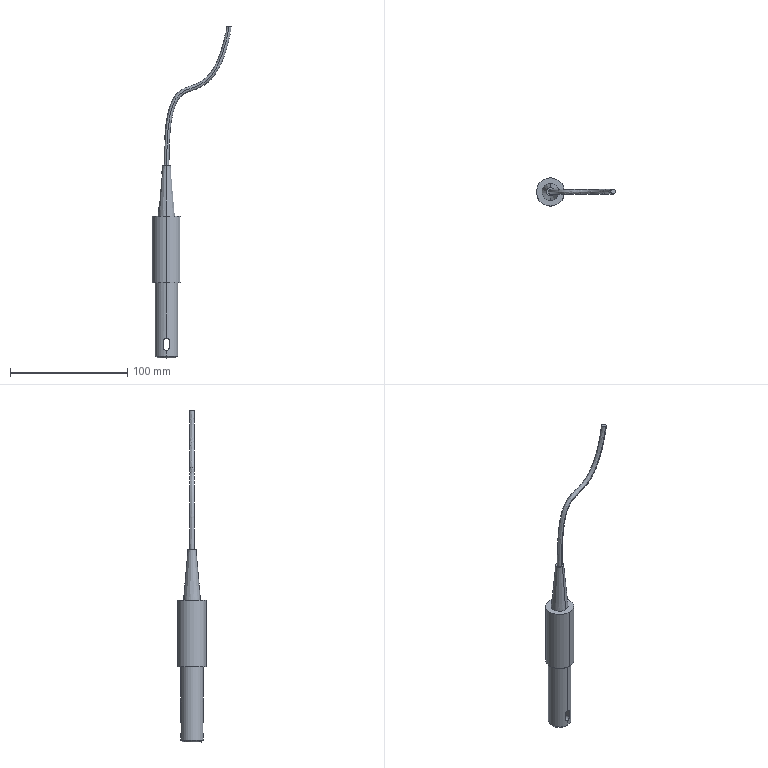Part | SolidWorks | features BaseBody 4 | 4 solids | 33 faces | box 67.479 x 24 x 282.859 mm | volume 49181 mm3 | plane 11 | cylinder 10 | spline 6 | cone 4 | torus 2 | commonest cylinder face diameters 0.32 x4 4.8 x2 19.2 x2 24 x2